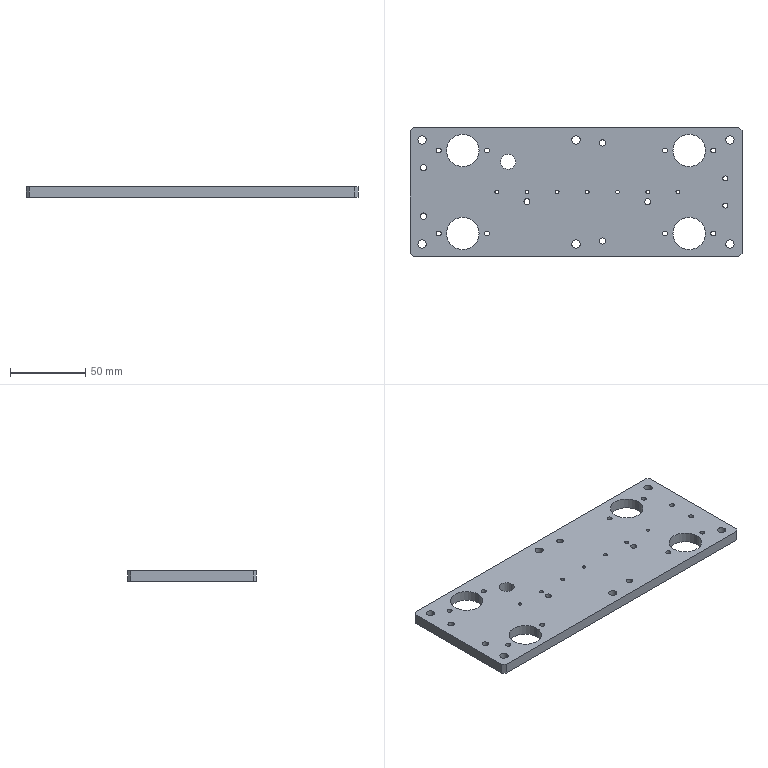Part | STEP file | PN_0036 | 1 solid | 78 faces | box 220 x 85 x 7 mm | volume 117728 mm3 | cylinder 68 | plane 10 | commonest cylinder face diameters 3.3 x20 2.5 x14 5.5 x12 4.2 x8 21.5 x8 4 x4